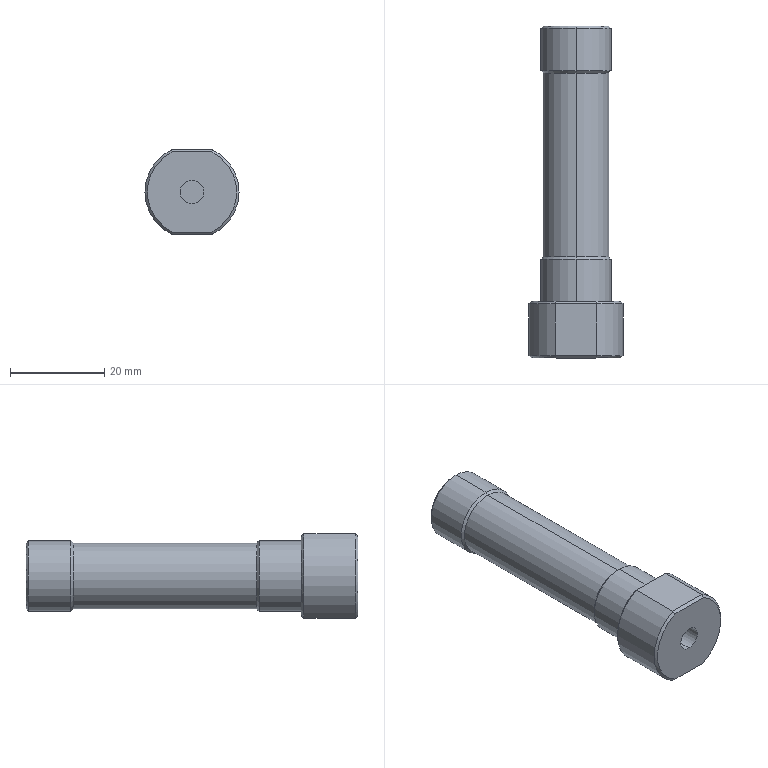Part | STEP file | ND25021-01-JDKM-13C-SL | 1 solid | 34 faces | box 20 x 70.5 x 18 mm | volume 12721 mm3 | cone 12 | cylinder 12 | plane 10 | commonest cylinder face diameters 15 x4 3.3 x2 5 x2 14 x2 20 x2